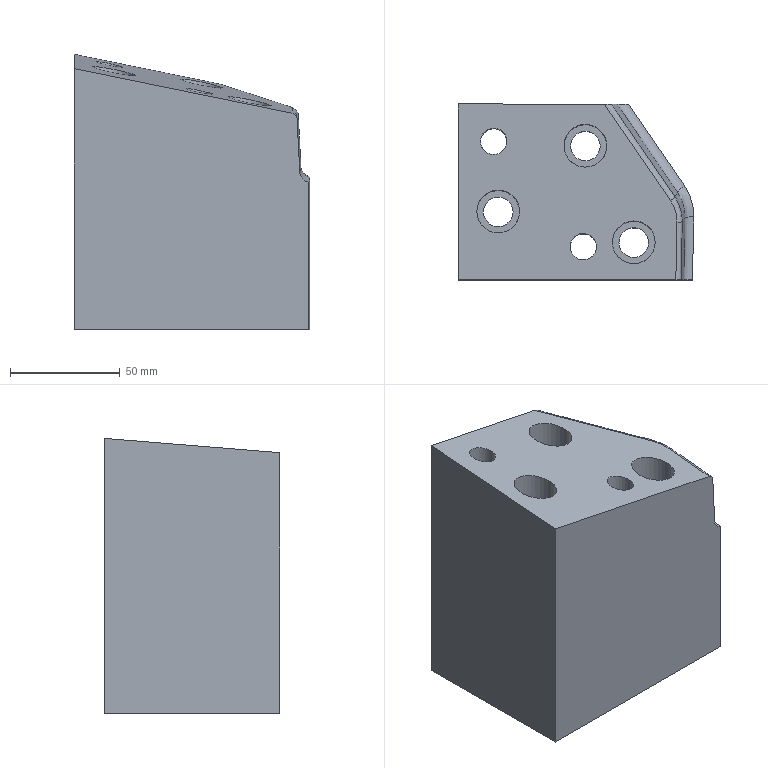Part | NX | features solid 2 | 1 solid | 28 faces | box 107.327 x 80 x 125.43 mm | volume 754575 mm3 | cylinder 10 | spline 9 | plane 9 | commonest cylinder face diameters 13.5 x3 19.5 x3 10 x2 12 x2
STEP:
#1=CARTESIAN_POINT('',(-857.279,-18.669,67.193));
#2=VERTEX_POINT('',#1);
#3=CARTESIAN_POINT('',(-859.902,-22.86,67.388));
#4=CARTESIAN_POINT('',(-856.633,-18.852,67.046));
#5=CARTESIAN_POINT('',(-857.243,-13.746,67.585));
#6=CARTESIAN_POINT('',(-861.169,-10.636,68.641));
#7=CARTESIAN_POINT('',(-866.18,-11.127,69.625));
#8=CARTESIAN_POINT('',(-869.446,-15.132,69.967));
#9=CARTESIAN_POINT('',(-868.843,-20.233,69.429));
#10=CARTESIAN_POINT('',(-864.913,-23.352,68.372));
#11=CARTESIAN_POINT('',(-859.902,-22.86,67.388));
#12=CARTESIAN_POINT('',(-856.633,-18.852,67.046));
#13=CARTESIAN_POINT('',(-857.243,-13.746,67.585));
#14=B_SPLINE_CURVE_WITH_KNOTS('',3,(#3,#4,#5,#6,#7,#8,#9,#10,#11,#12,#13),.UNSPECIFIED.,.T.,.F.,(1,1,1,1,1,1,1,1,1,1,1,1,1,1,1),(-0.01424,-0.009492,-0.004746,0.,0.004746,0.009492,0.01424,0.01898,0.02373,0.02848,0.03322,0.03797,0.04271,0.04746,0.05221),.UNSPECIFIED.);
#15=EDGE_CURVE('',#2,#2,#14,.T.);
#16=ORIENTED_EDGE('',*,*,#15,.F.);
#17=EDGE_LOOP('',(#16));
#18=FACE_BOUND('',#17,.T.);
#19=CARTESIAN_POINT('',(-909.709,-6.673,78.884));
#20=VERTEX_POINT('',#19);
#21=CARTESIAN_POINT('',(-903.612,-11.594,77.238));
#22=CARTESIAN_POINT('',(-910.538,-7.306,79.002));
#23=CARTESIAN_POINT('',(-912.489,0.7824,80.058));
#24=CARTESIAN_POINT('',(-908.008,7.886,79.719));
#25=CARTESIAN_POINT('',(-899.97,9.645,78.219));
#26=CARTESIAN_POINT('',(-893.065,5.359,76.46));
#27=CARTESIAN_POINT('',(-891.101,-2.711,75.402));
#28=CARTESIAN_POINT('',(-895.587,-9.835,75.74));
#29=CARTESIAN_POINT('',(-903.612,-11.594,77.238));
#30=CARTESIAN_POINT('',(-910.538,-7.306,79.002));
#31=CARTESIAN_POINT('',(-912.489,0.7824,80.058));
#32=B_SPLINE_CURVE_WITH_KNOTS('',3,(#21,#22,#23,#24,#25,#26,#27,#28,#29,#30,#31),.UNSPECIFIED.,.T.,.F.,(1,1,1,1,1,1,1,1,1,1,1,1,1,1,1),(-0.02314,-0.01542,-0.007712,0.,0.007712,0.01542,0.02314,0.03085,0.03856,0.04627,0.05398,0.06169,0.06941,0.07712,0.08483),.UNSPECIFIED.);
#33=EDGE_CURVE('',#20,#20,#32,.T.);
#34=ORIENTED_EDGE('',*,*,#33,.T.);
#35=EDGE_LOOP('',(#34));
#36=FACE_BOUND('',#35,.T.);
#37=CARTESIAN_POINT('',(-849.687,-16.103,65.849));
#38=VERTEX_POINT('',#37);
#39=CARTESIAN_POINT('',(-846.7,-23.44,64.643));
#40=CARTESIAN_POINT('',(-850.754,-16.253,66.055));
#41=CARTESIAN_POINT('',(-848.406,-8.168,66.232));
#42=CARTESIAN_POINT('',(-841.091,-4.27,65.054));
#43=CARTESIAN_POINT('',(-833.29,-6.567,63.273));
#44=CARTESIAN_POINT('',(-829.252,-13.743,61.864));
#45=CARTESIAN_POINT('',(-831.581,-21.819,61.684));
#46=CARTESIAN_POINT('',(-838.912,-25.731,62.864));
#47=CARTESIAN_POINT('',(-846.7,-23.44,64.643));
#48=CARTESIAN_POINT('',(-850.754,-16.253,66.055));
#49=CARTESIAN_POINT('',(-848.406,-8.168,66.232));
#50=B_SPLINE_CURVE_WITH_KNOTS('',3,(#39,#40,#41,#42,#43,#44,#45,#46,#47,#48,#49),.UNSPECIFIED.,.T.,.F.,(1,1,1,1,1,1,1,1,1,1,1,1,1,1,1),(-0.02314,-0.01543,-0.007713,0.,0.007713,0.01543,0.02314,0.03085,0.03857,0.04628,0.05399,0.06171,0.06942,0.07713,0.08485),.UNSPECIFIED.);
#51=EDGE_CURVE('',#38,#38,#50,.T.);
#52=ORIENTED_EDGE('',*,*,#51,.T.);
#53=EDGE_LOOP('',(#52));
#54=FACE_BOUND('',#53,.T.);
#55=CARTESIAN_POINT('',(-871.247,25.732,73.656));
#56=VERTEX_POINT('',#55);
#57=CARTESIAN_POINT('',(-866.719,19.289,72.207));
#58=CARTESIAN_POINT('',(-872.237,25.345,73.827));
#59=CARTESIAN_POINT('',(-871.815,33.724,74.421));
#60=CARTESIAN_POINT('',(-865.534,39.227,73.585));
#61=CARTESIAN_POINT('',(-857.389,38.706,71.878));
#62=CARTESIAN_POINT('',(-851.893,32.658,70.263));
#63=CARTESIAN_POINT('',(-852.296,24.292,69.666));
#64=CARTESIAN_POINT('',(-858.589,18.772,70.503));
#65=CARTESIAN_POINT('',(-866.719,19.289,72.207));
#66=CARTESIAN_POINT('',(-872.237,25.345,73.827));
#67=CARTESIAN_POINT('',(-871.815,33.724,74.421));
#68=B_SPLINE_CURVE_WITH_KNOTS('',3,(#57,#58,#59,#60,#61,#62,#63,#64,#65,#66,#67),.UNSPECIFIED.,.T.,.F.,(1,1,1,1,1,1,1,1,1,1,1,1,1,1,1),(-0.02314,-0.01543,-0.007713,0.,0.007713,0.01543,0.02314,0.03085,0.03856,0.04628,0.05399,0.0617,0.06942,0.07713,0.08484),.UNSPECIFIED.);
#69=EDGE_CURVE('',#56,#56,#68,.T.);
#70=ORIENTED_EDGE('',*,*,#69,.T.);
#71=EDGE_LOOP('',(#70));
#72=FACE_BOUND('',#71,.T.);
#73=CARTESIAN_POINT('',(-820.85,-32.,58.663));
#74=VERTEX_POINT('',#73);
#75=CARTESIAN_POINT('',(-920.,-32.,78.929));
#76=VERTEX_POINT('',#75);
#77=CARTESIAN_POINT('',(-820.85,-32.,58.663));
#78=CARTESIAN_POINT('',(-853.9,-32.,65.419));
#79=CARTESIAN_POINT('',(-886.95,-32.,72.174));
#80=CARTESIAN_POINT('',(-920.,-32.,78.929));
#81=B_SPLINE_CURVE_WITH_KNOTS('',3,(#77,#78,#79,#80),.UNSPECIFIED.,.F.,.F.,(4,4),(0.,0.1012),.UNSPECIFIED.);
#82=EDGE_CURVE('',#74,#76,#81,.T.);
#83=ORIENTED_EDGE('',*,*,#82,.F.);
#84=CARTESIAN_POINT('',(-820.322,-5.79,60.685));
#85=VERTEX_POINT('',#84);
#86=CARTESIAN_POINT('',(-820.85,-32.,58.663));
#87=CARTESIAN_POINT('',(-820.674,-23.263,59.337));
#88=CARTESIAN_POINT('',(-820.498,-14.527,60.011));
#89=CARTESIAN_POINT('',(-820.322,-5.79,60.685));
#90=B_SPLINE_CURVE_WITH_KNOTS('',3,(#86,#87,#88,#89),.UNSPECIFIED.,.F.,.F.,(4,4),(-0.002388,0.0239),.UNSPECIFIED.);
#91=EDGE_CURVE('',#74,#85,#90,.T.);
#92=ORIENTED_EDGE('',*,*,#91,.T.);
#93=CARTESIAN_POINT('',(-823.204,3.89,62.061));
#94=VERTEX_POINT('',#93);
#95=CARTESIAN_POINT('',(-820.322,-5.79,60.685));
#96=CARTESIAN_POINT('',(-820.252,-2.334,60.952));
#97=CARTESIAN_POINT('',(-821.278,1.075,61.439));
#98=CARTESIAN_POINT('',(-823.204,3.89,62.061));
#99=B_SPLINE_CURVE_WITH_KNOTS('',3,(#95,#96,#97,#98),.UNSPECIFIED.,.F.,.F.,(4,4),(0.,0.01034),.UNSPECIFIED.);
#100=EDGE_CURVE('',#85,#94,#99,.T.);
#101=ORIENTED_EDGE('',*,*,#100,.T.);
#102=CARTESIAN_POINT('',(-853.376,48.,71.813));
#103=VERTEX_POINT('',#102);
#104=CARTESIAN_POINT('',(-823.204,3.89,62.061));
#105=CARTESIAN_POINT('',(-833.261,18.593,65.312));
#106=CARTESIAN_POINT('',(-843.319,33.297,68.562));
#107=CARTESIAN_POINT('',(-853.376,48.,71.813));
#108=B_SPLINE_CURVE_WITH_KNOTS('',3,(#104,#105,#106,#107),.UNSPECIFIED.,.F.,.F.,(4,4),(0.,0.05432),.UNSPECIFIED.);
#109=EDGE_CURVE('',#94,#103,#108,.T.);
#110=ORIENTED_EDGE('',*,*,#109,.T.);
#111=CARTESIAN_POINT('',(-920.,48.,85.43));
#112=VERTEX_POINT('',#111);
#113=CARTESIAN_POINT('',(-853.376,48.,71.813));
#114=CARTESIAN_POINT('',(-875.584,48.,76.352));
#115=CARTESIAN_POINT('',(-897.792,48.,80.891));
#116=CARTESIAN_POINT('',(-920.,48.,85.43));
#117=B_SPLINE_CURVE_WITH_KNOTS('',3,(#113,#114,#115,#116),.UNSPECIFIED.,.F.,.F.,(4,4),(0.1961,0.2641),.UNSPECIFIED.);
#118=EDGE_CURVE('',#103,#112,#117,.T.);
#119=ORIENTED_EDGE('',*,*,#118,.T.);
#120=CARTESIAN_POINT('',(-920.,-32.,78.929));
#121=CARTESIAN_POINT('',(-920.,-5.333,81.096));
#122=CARTESIAN_POINT('',(-920.,21.333,83.263));
#123=CARTESIAN_POINT('',(-920.,48.,85.43));
#124=B_SPLINE_CURVE_WITH_KNOTS('',3,(#120,#121,#122,#123),.UNSPECIFIED.,.F.,.F.,(4,4),(0.,0.08026),.UNSPECIFIED.);
#125=EDGE_CURVE('',#76,#112,#124,.T.);
#126=ORIENTED_EDGE('',*,*,#125,.F.);
#127=EDGE_LOOP('',(#83,#92,#101,#110,#119,#126));
#128=FACE_BOUND('',#127,.T.);
#129=CARTESIAN_POINT('',(-908.757,34.366,82.024));
#130=VERTEX_POINT('',#129);
#131=CARTESIAN_POINT('',(-904.976,37.499,81.506));
#132=CARTESIAN_POINT('',(-909.304,34.754,82.168));
#133=CARTESIAN_POINT('',(-910.352,29.683,81.97));
#134=CARTESIAN_POINT('',(-907.547,25.48,81.055));
#135=CARTESIAN_POINT('',(-902.655,24.423,79.969));
#136=CARTESIAN_POINT('',(-898.335,27.166,79.309));
#137=CARTESIAN_POINT('',(-897.28,32.228,79.505));
#138=CARTESIAN_POINT('',(-900.089,36.443,80.421));
#139=CARTESIAN_POINT('',(-904.976,37.499,81.506));
#140=CARTESIAN_POINT('',(-909.304,34.754,82.168));
#141=CARTESIAN_POINT('',(-910.352,29.683,81.97));
#142=B_SPLINE_CURVE_WITH_KNOTS('',3,(#131,#132,#133,#134,#135,#136,#137,#138,#139,#140,#141),.UNSPECIFIED.,.T.,.F.,(1,1,1,1,1,1,1,1,1,1,1,1,1,1,1),(-0.01424,-0.009493,-0.004747,0.,0.004747,0.009493,0.01424,0.01899,0.02373,0.02848,0.03323,0.03797,0.04272,0.04747,0.05221),.UNSPECIFIED.);
#143=EDGE_CURVE('',#130,#130,#142,.T.);
#144=ORIENTED_EDGE('',*,*,#143,.F.);
#145=EDGE_LOOP('',(#144));
#146=FACE_BOUND('',#145,.T.);
#147=CARTESIAN_POINT('',(-920.973,48.472,85.668));
#148=CARTESIAN_POINT('',(-920.587,-34.619,78.836));
#149=CARTESIAN_POINT('',(-919.909,48.495,85.452));
#150=CARTESIAN_POINT('',(-919.523,-34.596,78.62));
#151=CARTESIAN_POINT('',(-900.858,48.901,81.591));
#152=CARTESIAN_POINT('',(-900.471,-34.19,74.759));
#153=CARTESIAN_POINT('',(-869.11,49.577,75.157));
#154=CARTESIAN_POINT('',(-868.723,-33.513,68.325));
#155=CARTESIAN_POINT('',(-819.956,50.625,65.195));
#156=CARTESIAN_POINT('',(-819.569,-32.465,58.364));
#157=B_SPLINE_SURFACE_WITH_KNOTS('',1,1,((#147,#148),(#149,#150),(#151,#152),(#153,#154),(#155,#156)),.PLANE_SURF.,.F.,.F.,.F.,(2,1,1,1,2),(2,2),(-0.2849,-0.2791,-0.1744,0.,0.2701),(0.3913,0.7679),.PIECEWISE_BEZIER_KNOTS.);
#158=ADVANCED_FACE('',(#18,#36,#54,#72,#128,#146),#157,.F.);
#159=CARTESIAN_POINT('',(-869.041,-16.993,-40.));
#160=VERTEX_POINT('',#159);
#161=CARTESIAN_POINT('',(-863.041,-16.993,-40.));
#162=DIRECTION('',(0.,0.,-1.));
#163=DIRECTION('',(-1.,0.,0.));
#164=AXIS2_PLACEMENT_3D('',#161,#162,#163);
#165=CIRCLE('',#164,6.);
#166=EDGE_CURVE('',#160,#160,#165,.F.);
#167=ORIENTED_EDGE('',*,*,#166,.T.);
#168=EDGE_LOOP('',(#167));
#169=FACE_BOUND('',#168,.T.);
#170=CARTESIAN_POINT('',(-908.547,-0.9737,-40.));
#171=VERTEX_POINT('',#170);
#172=CARTESIAN_POINT('',(-901.797,-0.9737,-40.));
#173=DIRECTION('',(0.,0.,-1.));
#174=DIRECTION('',(-1.,0.,0.));
#175=AXIS2_PLACEMENT_3D('',#172,#173,#174);
#176=CIRCLE('',#175,6.75);
#177=EDGE_CURVE('',#171,#171,#176,.T.);
#178=ORIENTED_EDGE('',*,*,#177,.F.);
#179=EDGE_LOOP('',(#178));
#180=FACE_BOUND('',#179,.T.);
#181=CARTESIAN_POINT('',(-846.75,-15.,-40.));
#182=VERTEX_POINT('',#181);
#183=CARTESIAN_POINT('',(-840.,-15.,-40.));
#184=DIRECTION('',(0.,0.,-1.));
#185=DIRECTION('',(-1.,0.,0.));
#186=AXIS2_PLACEMENT_3D('',#183,#184,#185);
#187=CIRCLE('',#186,6.75);
#188=EDGE_CURVE('',#182,#182,#187,.T.);
#189=ORIENTED_EDGE('',*,*,#188,.F.);
#190=EDGE_LOOP('',(#189));
#191=FACE_BOUND('',#190,.T.);
#192=CARTESIAN_POINT('',(-868.811,29.,-40.));
#193=VERTEX_POINT('',#192);
#194=CARTESIAN_POINT('',(-862.061,29.,-40.));
#195=DIRECTION('',(0.,0.,-1.));
#196=DIRECTION('',(-1.,0.,0.));
#197=AXIS2_PLACEMENT_3D('',#194,#195,#196);
#198=CIRCLE('',#197,6.75);
#199=EDGE_CURVE('',#193,#193,#198,.T.);
#200=ORIENTED_EDGE('',*,*,#199,.F.);
#201=EDGE_LOOP('',(#200));
#202=FACE_BOUND('',#201,.T.);
#203=CARTESIAN_POINT('',(-813.255,-32.,-40.));
#204=VERTEX_POINT('',#203);
#205=CARTESIAN_POINT('',(-920.,-32.,-40.));
#206=VERTEX_POINT('',#205);
#207=CARTESIAN_POINT('',(-813.69,-32.,-40.));
#208=DIRECTION('',(-1.,0.,0.));
#209=VECTOR('',#208,1000.);
#210=LINE('',#207,#209);
#211=EDGE_CURVE('',#204,#206,#210,.T.);
#212=ORIENTED_EDGE('',*,*,#211,.T.);
#213=CARTESIAN_POINT('',(-920.,48.,-40.));
#214=VERTEX_POINT('',#213);
#215=CARTESIAN_POINT('',(-920.,-31.695,-40.));
#216=DIRECTION('',(0.,1.,0.));
#217=VECTOR('',#216,1000.);
#218=LINE('',#215,#217);
#219=EDGE_CURVE('',#206,#214,#218,.T.);
#220=ORIENTED_EDGE('',*,*,#219,.T.);
#221=CARTESIAN_POINT('',(-842.318,48.,-40.));
#222=VERTEX_POINT('',#221);
#223=CARTESIAN_POINT('',(-813.69,48.,-40.));
#224=DIRECTION('',(1.,0.,0.));
#225=VECTOR('',#224,1000.);
#226=LINE('',#223,#225);
#227=EDGE_CURVE('',#222,#214,#226,.F.);
#228=ORIENTED_EDGE('',*,*,#227,.F.);
#229=CARTESIAN_POINT('',(-816.916,10.864,-40.));
#230=VERTEX_POINT('',#229);
#231=CARTESIAN_POINT('',(-812.737,4.755,-40.));
#232=DIRECTION('',(0.5646,-0.8254,0.));
#233=VECTOR('',#232,1000.);
#234=LINE('',#231,#233);
#235=EDGE_CURVE('',#222,#230,#234,.T.);
#236=ORIENTED_EDGE('',*,*,#235,.T.);
#237=CARTESIAN_POINT('',(-812.678,-3.372,-40.));
#238=VERTEX_POINT('',#237);
#239=CARTESIAN_POINT('',(-812.678,-3.372,-40.));
#240=CARTESIAN_POINT('',(-812.627,-0.8443,-40.));
#241=CARTESIAN_POINT('',(-813.295,4.147,-40.));
#242=CARTESIAN_POINT('',(-815.489,8.778,-40.));
#243=CARTESIAN_POINT('',(-816.916,10.864,-40.));
#244=B_SPLINE_CURVE_WITH_KNOTS('',3,(#239,#240,#241,#242,#243),.UNSPECIFIED.,.F.,.F.,(4,1,4),(0.06077,0.06835,0.07594),.UNSPECIFIED.);
#245=EDGE_CURVE('',#238,#230,#244,.T.);
#246=ORIENTED_EDGE('',*,*,#245,.F.);
#247=CARTESIAN_POINT('',(-812.528,4.08,-40.));
#248=DIRECTION('',(0.02015,0.9998,0.));
#249=VECTOR('',#248,1000.);
#250=LINE('',#247,#249);
#251=EDGE_CURVE('',#204,#238,#250,.T.);
#252=ORIENTED_EDGE('',*,*,#251,.F.);
#253=EDGE_LOOP('',(#212,#220,#228,#236,#246,#252));
#254=FACE_BOUND('',#253,.T.);
#255=CARTESIAN_POINT('',(-909.818,30.961,-40.));
#256=VERTEX_POINT('',#255);
#257=CARTESIAN_POINT('',(-903.818,30.961,-40.));
#258=DIRECTION('',(0.,0.,-1.));
#259=DIRECTION('',(-1.,0.,0.));
#260=AXIS2_PLACEMENT_3D('',#257,#258,#259);
#261=CIRCLE('',#260,6.);
#262=EDGE_CURVE('',#256,#256,#261,.F.);
#263=ORIENTED_EDGE('',*,*,#262,.T.);
#264=EDGE_LOOP('',(#263));
#265=FACE_BOUND('',#264,.T.);
#266=CARTESIAN_POINT('',(-813.69,4.103,-40.));
#267=DIRECTION('',(0.,0.,-1.));
#268=DIRECTION('',(-1.,0.,0.));
#269=AXIS2_PLACEMENT_3D('',#266,#267,#268);
#270=PLANE('',#269);
#271=ADVANCED_FACE('',(#169,#180,#191,#202,#254,#265),#270,.T.);
#272=CARTESIAN_POINT('',(-818.457,-32.,55.871));
#273=VERTEX_POINT('',#272);
#274=CARTESIAN_POINT('',(-817.244,-32.,31.764));
#275=VERTEX_POINT('',#274);
#276=CARTESIAN_POINT('',(-818.457,-32.,55.871));
#277=CARTESIAN_POINT('',(-818.053,-32.,47.836));
#278=CARTESIAN_POINT('',(-817.648,-32.,39.8));
#279=CARTESIAN_POINT('',(-817.244,-32.,31.764));
#280=B_SPLINE_CURVE_WITH_KNOTS('',3,(#276,#277,#278,#279),.UNSPECIFIED.,.F.,.F.,(4,4),(0.06257,0.08671),.UNSPECIFIED.);
#281=EDGE_CURVE('',#273,#275,#280,.T.);
#282=ORIENTED_EDGE('',*,*,#281,.F.);
#283=CARTESIAN_POINT('',(-818.457,-32.,55.871));
#284=CARTESIAN_POINT('',(-818.524,-32.,57.201));
#285=CARTESIAN_POINT('',(-819.546,-32.,58.397));
#286=CARTESIAN_POINT('',(-820.85,-32.,58.663));
#287=B_SPLINE_CURVE_WITH_KNOTS('',3,(#283,#284,#285,#286),.UNSPECIFIED.,.F.,.F.,(4,4),(0.,0.003938),.UNSPECIFIED.);
#288=EDGE_CURVE('',#273,#74,#287,.T.);
#289=ORIENTED_EDGE('',*,*,#288,.T.);
#290=ORIENTED_EDGE('',*,*,#82,.T.);
#291=CARTESIAN_POINT('',(-920.,-32.,100.));
#292=DIRECTION('',(0.,0.,-1.));
#293=VECTOR('',#292,1000.);
#294=LINE('',#291,#293);
#295=EDGE_CURVE('',#76,#206,#294,.T.);
#296=ORIENTED_EDGE('',*,*,#295,.T.);
#297=ORIENTED_EDGE('',*,*,#211,.F.);
#298=CARTESIAN_POINT('',(-813.255,-32.,27.111));
#299=VERTEX_POINT('',#298);
#300=CARTESIAN_POINT('',(-813.255,-32.,-47.5));
#301=DIRECTION('',(0.,0.,-1.));
#302=VECTOR('',#301,1000.);
#303=LINE('',#300,#302);
#304=EDGE_CURVE('',#299,#204,#303,.T.);
#305=ORIENTED_EDGE('',*,*,#304,.F.);
#306=CARTESIAN_POINT('',(-812.249,-32.,32.025));
#307=DIRECTION('',(0.,-1.,0.));
#308=DIRECTION('',(0.2528,0.,0.9675));
#309=AXIS2_PLACEMENT_3D('',#306,#307,#308);
#310=ELLIPSE('',#309,5.016,5.);
#311=EDGE_CURVE('',#299,#275,#310,.F.);
#312=ORIENTED_EDGE('',*,*,#311,.T.);
#313=EDGE_LOOP('',(#282,#289,#290,#296,#297,#305,#312));
#314=FACE_BOUND('',#313,.T.);
#315=CARTESIAN_POINT('',(-915.5,-32.,-47.5));
#316=DIRECTION('',(0.,-1.,0.));
#317=DIRECTION('',(1.,0.,0.));
#318=AXIS2_PLACEMENT_3D('',#315,#316,#317);
#319=PLANE('',#318);
#320=ADVANCED_FACE('',(#314),#319,.T.);
#321=ORIENTED_EDGE('',*,*,#118,.F.);
#322=CARTESIAN_POINT('',(-850.193,48.,68.733));
#323=VERTEX_POINT('',#322);
#324=CARTESIAN_POINT('',(-853.376,48.,71.813));
#325=CARTESIAN_POINT('',(-852.599,48.,71.654));
#326=CARTESIAN_POINT('',(-851.151,48.,70.951));
#327=CARTESIAN_POINT('',(-850.277,48.,69.525));
#328=CARTESIAN_POINT('',(-850.193,48.,68.733));
#329=B_SPLINE_CURVE_WITH_KNOTS('',3,(#324,#325,#326,#327,#328),.UNSPECIFIED.,.F.,.F.,(4,1,4),(0.,0.002346,0.004693),.UNSPECIFIED.);
#330=EDGE_CURVE('',#103,#323,#329,.T.);
#331=ORIENTED_EDGE('',*,*,#330,.T.);
#332=CARTESIAN_POINT('',(-847.625,48.,44.687));
#333=VERTEX_POINT('',#332);
#334=CARTESIAN_POINT('',(-847.625,48.,44.687));
#335=CARTESIAN_POINT('',(-848.481,48.,52.702));
#336=CARTESIAN_POINT('',(-849.337,48.,60.717));
#337=CARTESIAN_POINT('',(-850.193,48.,68.733));
#338=B_SPLINE_CURVE_WITH_KNOTS('',3,(#334,#335,#336,#337),.UNSPECIFIED.,.F.,.F.,(4,4),(0.,0.02418),.UNSPECIFIED.);
#339=EDGE_CURVE('',#333,#323,#338,.T.);
#340=ORIENTED_EDGE('',*,*,#339,.F.);
#341=CARTESIAN_POINT('',(-842.318,48.,39.553));
#342=VERTEX_POINT('',#341);
#343=CARTESIAN_POINT('',(-841.592,48.,44.524));
#344=DIRECTION('',(0.,1.,0.));
#345=DIRECTION('',(0.9515,0.,-0.3075));
#346=AXIS2_PLACEMENT_3D('',#343,#344,#345);
#347=ELLIPSE('',#346,6.158,5.);
#348=EDGE_CURVE('',#342,#333,#347,.T.);
#349=ORIENTED_EDGE('',*,*,#348,.F.);
#350=CARTESIAN_POINT('',(-842.318,48.,100.));
#351=DIRECTION('',(0.,0.,1.));
#352=VECTOR('',#351,1000.);
#353=LINE('',#350,#352);
#354=EDGE_CURVE('',#342,#222,#353,.F.);
#355=ORIENTED_EDGE('',*,*,#354,.T.);
#356=ORIENTED_EDGE('',*,*,#227,.T.);
#357=CARTESIAN_POINT('',(-920.,48.,100.));
#358=DIRECTION('',(0.,0.,1.));
#359=VECTOR('',#358,1000.);
#360=LINE('',#357,#359);
#361=EDGE_CURVE('',#112,#214,#360,.F.);
#362=ORIENTED_EDGE('',*,*,#361,.F.);
#363=EDGE_LOOP('',(#321,#331,#340,#349,#355,#356,#362));
#364=FACE_BOUND('',#363,.T.);
#365=CARTESIAN_POINT('',(-915.5,48.,-47.5));
#366=DIRECTION('',(0.,1.,0.));
#367=DIRECTION('',(-1.,0.,0.));
#368=AXIS2_PLACEMENT_3D('',#365,#366,#367);
#369=PLANE('',#368);
#370=ADVANCED_FACE('',(#364),#369,.T.);
#371=ORIENTED_EDGE('',*,*,#354,.F.);
#372=CARTESIAN_POINT('',(-816.916,10.864,31.343));
#373=VERTEX_POINT('',#372);
#374=CARTESIAN_POINT('',(-842.318,48.,39.553));
#375=CARTESIAN_POINT('',(-833.851,35.621,36.816));
#376=CARTESIAN_POINT('',(-825.383,23.243,34.079));
#377=CARTESIAN_POINT('',(-816.916,10.864,31.343));
#378=B_SPLINE_CURVE_WITH_KNOTS('',3,(#374,#375,#376,#377),.UNSPECIFIED.,.F.,.F.,(4,4),(-0.01765,1.),.UNSPECIFIED.);
#379=EDGE_CURVE('',#342,#373,#378,.T.);
#380=ORIENTED_EDGE('',*,*,#379,.T.);
#381=CARTESIAN_POINT('',(-816.916,10.864,100.));
#382=DIRECTION('',(0.,0.,-1.));
#383=VECTOR('',#382,1000.);
#384=LINE('',#381,#383);
#385=EDGE_CURVE('',#373,#230,#384,.T.);
#386=ORIENTED_EDGE('',*,*,#385,.T.);
#387=ORIENTED_EDGE('',*,*,#235,.F.);
#388=EDGE_LOOP('',(#371,#380,#386,#387));
#389=FACE_BOUND('',#388,.T.);
#390=CARTESIAN_POINT('',(-841.878,47.356,100.));
#391=DIRECTION('',(0.8254,0.5646,0.));
#392=DIRECTION('',(-0.5646,0.8254,0.));
#393=AXIS2_PLACEMENT_3D('',#390,#391,#392);
#394=PLANE('',#393);
#395=ADVANCED_FACE('',(#389),#394,.T.);
#396=CARTESIAN_POINT('',(-812.678,-3.372,29.32));
#397=VERTEX_POINT('',#396);
#398=CARTESIAN_POINT('',(-813.255,-32.,27.111));
#399=CARTESIAN_POINT('',(-813.063,-22.457,27.847));
#400=CARTESIAN_POINT('',(-812.87,-12.914,28.583));
#401=CARTESIAN_POINT('',(-812.678,-3.372,29.32));
#402=B_SPLINE_CURVE_WITH_KNOTS('',3,(#398,#399,#400,#401),.UNSPECIFIED.,.F.,.F.,(4,4),(-0.0907,1.),.UNSPECIFIED.);
#403=EDGE_CURVE('',#299,#397,#402,.T.);
#404=ORIENTED_EDGE('',*,*,#403,.F.);
#405=ORIENTED_EDGE('',*,*,#304,.T.);
#406=ORIENTED_EDGE('',*,*,#251,.T.);
#407=CARTESIAN_POINT('',(-812.678,-3.372,100.));
#408=DIRECTION('',(0.,0.,-1.));
#409=VECTOR('',#408,1000.);
#410=LINE('',#407,#409);
#411=EDGE_CURVE('',#397,#238,#410,.T.);
#412=ORIENTED_EDGE('',*,*,#411,.F.);
#413=EDGE_LOOP('',(#404,#405,#406,#412));
#414=FACE_BOUND('',#413,.T.);
#415=CARTESIAN_POINT('',(-813.207,-29.619,100.));
#416=DIRECTION('',(-0.9998,0.02015,0.));
#417=DIRECTION('',(-0.02015,-0.9998,0.));
#418=AXIS2_PLACEMENT_3D('',#415,#416,#417);
#419=PLANE('',#418);
#420=ADVANCED_FACE('',(#414),#419,.F.);
#421=ORIENTED_EDGE('',*,*,#219,.F.);
#422=ORIENTED_EDGE('',*,*,#295,.F.);
#423=ORIENTED_EDGE('',*,*,#125,.T.);
#424=ORIENTED_EDGE('',*,*,#361,.T.);
#425=EDGE_LOOP('',(#421,#422,#423,#424));
#426=FACE_BOUND('',#425,.T.);
#427=CARTESIAN_POINT('',(-920.,-31.695,100.));
#428=DIRECTION('',(1.,0.,0.));
#429=DIRECTION('',(0.,0.,1.));
#430=AXIS2_PLACEMENT_3D('',#427,#428,#429);
#431=PLANE('',#430);
#432=ADVANCED_FACE('',(#426),#431,.F.);
#433=ORIENTED_EDGE('',*,*,#385,.F.);
#434=CARTESIAN_POINT('',(-816.916,10.864,31.343));
#435=CARTESIAN_POINT('',(-813.844,6.373,30.35));
#436=CARTESIAN_POINT('',(-812.585,1.24,29.675));
#437=CARTESIAN_POINT('',(-812.678,-3.372,29.32));
#438=B_SPLINE_CURVE_WITH_KNOTS('',3,(#434,#435,#436,#437),.UNSPECIFIED.,.F.,.F.,(4,4),(0.,1.),.UNSPECIFIED.);
#439=EDGE_CURVE('',#373,#397,#438,.T.);
#440=ORIENTED_EDGE('',*,*,#439,.T.);
#441=ORIENTED_EDGE('',*,*,#411,.T.);
#442=ORIENTED_EDGE('',*,*,#245,.T.);
#443=EDGE_LOOP('',(#433,#440,#441,#442));
#444=FACE_BOUND('',#443,.T.);
#445=CARTESIAN_POINT('',(-812.678,-3.372,31.771));
#446=CARTESIAN_POINT('',(-812.678,-3.372,-40.));
#447=CARTESIAN_POINT('',(-812.576,1.691,31.771));
#448=CARTESIAN_POINT('',(-812.576,1.691,-40.));
#449=CARTESIAN_POINT('',(-814.095,6.74,31.771));
#450=CARTESIAN_POINT('',(-814.095,6.74,-40.));
#451=CARTESIAN_POINT('',(-816.916,10.864,31.771));
#452=CARTESIAN_POINT('',(-816.916,10.864,-40.));
#453=B_SPLINE_SURFACE_WITH_KNOTS('',3,1,((#445,#446),(#447,#448),(#449,#450),(#451,#452)),.SURF_OF_LINEAR_EXTRUSION.,.F.,.F.,.F.,(4,4),(2,2),(0.,1.),(0.,1.),.PIECEWISE_BEZIER_KNOTS.);
#454=ADVANCED_FACE('',(#444),#453,.F.);
#455=ORIENTED_EDGE('',*,*,#348,.T.);
#456=CARTESIAN_POINT('',(-844.632,43.625,43.72));
#457=VERTEX_POINT('',#456);
#458=CARTESIAN_POINT('',(-813.552,-1.812,33.674));
#459=DIRECTION('',(0.5554,-0.812,-0.1795));
#460=VECTOR('',#459,1000.);
#461=LINE('',#458,#460);
#462=EDGE_CURVE('',#457,#333,#461,.F.);
#463=ORIENTED_EDGE('',*,*,#462,.F.);
#464=CARTESIAN_POINT('',(-820.074,7.722,35.782));
#465=VERTEX_POINT('',#464);
#466=CARTESIAN_POINT('',(-820.074,7.722,35.782));
#467=CARTESIAN_POINT('',(-828.26,19.69,38.428));
#468=CARTESIAN_POINT('',(-836.446,31.657,41.074));
#469=CARTESIAN_POINT('',(-844.632,43.625,43.72));
#470=B_SPLINE_CURVE_WITH_KNOTS('',3,(#466,#467,#468,#469),.UNSPECIFIED.,.F.,.F.,(4,4),(0.,1.),.UNSPECIFIED.);
#471=EDGE_CURVE('',#465,#457,#470,.T.);
#472=ORIENTED_EDGE('',*,*,#471,.F.);
#473=CARTESIAN_POINT('',(-816.916,10.864,31.343));
#474=CARTESIAN_POINT('',(-817.831,10.208,31.476));
#475=CARTESIAN_POINT('',(-819.497,8.836,32.526));
#476=CARTESIAN_POINT('',(-820.104,7.947,34.672));
#477=CARTESIAN_POINT('',(-820.074,7.722,35.782));
#478=B_SPLINE_CURVE_WITH_KNOTS('',3,(#473,#474,#475,#476,#477),.UNSPECIFIED.,.F.,.F.,(4,1,4),(0.,0.5,1.),.UNSPECIFIED.);
#479=EDGE_CURVE('',#465,#373,#478,.F.);
#480=ORIENTED_EDGE('',*,*,#479,.T.);
#481=ORIENTED_EDGE('',*,*,#379,.F.);
#482=EDGE_LOOP('',(#455,#463,#472,#480,#481));
#483=FACE_BOUND('',#482,.T.);
#484=CARTESIAN_POINT('',(-809.396,0.9322,34.118));
#485=DIRECTION('',(0.5554,-0.812,-0.1795));
#486=DIRECTION('',(-0.8312,-0.5489,-0.08875));
#487=AXIS2_PLACEMENT_3D('',#484,#485,#486);
#488=CYLINDRICAL_SURFACE('',#487,5.);
#489=ADVANCED_FACE('',(#483),#488,.F.);
#490=CARTESIAN_POINT('',(-821.309,5.775,59.397));
#491=VERTEX_POINT('',#490);
#492=CARTESIAN_POINT('',(-819.624,8.431,27.186));
#493=CARTESIAN_POINT('',(-819.845,8.082,31.423));
#494=CARTESIAN_POINT('',(-820.016,7.813,34.682));
#495=CARTESIAN_POINT('',(-821.153,6.021,56.409));
#496=CARTESIAN_POINT('',(-821.323,5.753,59.668));
#497=CARTESIAN_POINT('',(-821.545,5.403,63.905));
#498=(BOUNDED_CURVE()B_SPLINE_CURVE(1,(#492,#493,#494,#495,#496,#497),.UNSPECIFIED.,.F.,.F.)B_SPLINE_CURVE_WITH_KNOTS((2,1,1,1,1,2),(-0.345,-0.15,0.,1.,1.15,1.345),.PIECEWISE_BEZIER_KNOTS.)CURVE()GEOMETRIC_REPRESENTATION_ITEM()RATIONAL_B_SPLINE_CURVE((1.,1.,1.,1.,1.,1.))REPRESENTATION_ITEM(''));
#499=EDGE_CURVE('',#465,#491,#498,.T.);
#500=ORIENTED_EDGE('',*,*,#499,.T.);
#501=CARTESIAN_POINT('',(-817.926,-5.624,57.906));
#502=VERTEX_POINT('',#501);
#503=CARTESIAN_POINT('',(-821.309,5.775,59.397));
#504=CARTESIAN_POINT('',(-819.061,2.474,58.755));
#505=CARTESIAN_POINT('',(-817.844,-1.592,58.221));
#506=CARTESIAN_POINT('',(-817.926,-5.624,57.906));
#507=B_SPLINE_CURVE_WITH_KNOTS('',3,(#503,#504,#505,#506),.UNSPECIFIED.,.F.,.F.,(4,4),(-0.00000006,0.01214),.UNSPECIFIED.);
#508=EDGE_CURVE('',#491,#502,#507,.T.);
#509=ORIENTED_EDGE('',*,*,#508,.T.);
#510=CARTESIAN_POINT('',(-816.672,-3.648,33.952));
#511=VERTEX_POINT('',#510);
#512=CARTESIAN_POINT('',(-818.227,-6.099,63.671));
#513=CARTESIAN_POINT('',(-817.961,-5.679,58.575));
#514=CARTESIAN_POINT('',(-817.755,-5.356,54.656));
#515=CARTESIAN_POINT('',(-817.598,-5.107,51.641));
#516=CARTESIAN_POINT('',(-817.476,-4.916,49.322));
#517=CARTESIAN_POINT('',(-816.667,-3.641,33.86));
#518=CARTESIAN_POINT('',(-816.546,-3.45,31.541));
#519=CARTESIAN_POINT('',(-816.388,-3.201,28.526));
#520=CARTESIAN_POINT('',(-816.183,-2.878,24.606));
#521=CARTESIAN_POINT('',(-815.917,-2.458,19.511));
#522=B_SPLINE_CURVE_WITH_KNOTS('',1,(#512,#513,#514,#515,#516,#517,#518,#519,#520,#521),.UNSPECIFIED.,.F.,.F.,(2,1,1,1,1,1,1,1,1,2),(-0.9281,-0.5985,-0.345,-0.15,0.,1.,1.15,1.345,1.599,1.928),.PIECEWISE_BEZIER_KNOTS.);
#523=EDGE_CURVE('',#502,#511,#522,.T.);
#524=ORIENTED_EDGE('',*,*,#523,.T.);
#525=CARTESIAN_POINT('',(-816.672,-3.648,33.952));
#526=CARTESIAN_POINT('',(-816.595,0.1523,34.239));
#527=CARTESIAN_POINT('',(-817.731,4.321,34.88));
#528=CARTESIAN_POINT('',(-820.074,7.722,35.782));
#529=B_SPLINE_CURVE_WITH_KNOTS('',3,(#525,#526,#527,#528),.UNSPECIFIED.,.F.,.F.,(4,4),(0.,1.),.UNSPECIFIED.);
#530=EDGE_CURVE('',#511,#465,#529,.T.);
#531=ORIENTED_EDGE('',*,*,#530,.T.);
#532=EDGE_LOOP('',(#500,#509,#524,#531));
#533=FACE_BOUND('',#532,.T.);
#534=CARTESIAN_POINT('',(-816.67,-3.645,33.912));
#535=CARTESIAN_POINT('',(-817.807,-5.437,55.639));
#536=CARTESIAN_POINT('',(-818.091,-5.885,61.067));
#537=CARTESIAN_POINT('',(-816.589,0.4523,34.254));
#538=CARTESIAN_POINT('',(-817.726,-1.339,55.981));
#539=CARTESIAN_POINT('',(-818.01,-1.787,61.409));
#540=CARTESIAN_POINT('',(-817.739,4.392,34.519));
#541=CARTESIAN_POINT('',(-818.876,2.6,56.246));
#542=CARTESIAN_POINT('',(-819.16,2.153,61.674));
#543=CARTESIAN_POINT('',(-820.016,7.813,34.682));
#544=CARTESIAN_POINT('',(-821.153,6.021,56.409));
#545=CARTESIAN_POINT('',(-821.437,5.574,61.837));
#546=(BOUNDED_SURFACE()B_SPLINE_SURFACE(3,1,((#534,#535,#536),(#537,#538,#539),(#540,#541,#542),(#543,#544,#545)),.CYLINDRICAL_SURF.,.F.,.F.,.F.)B_SPLINE_SURFACE_WITH_KNOTS((4,4),(2,1,2),(0.,1.),(0.,1.,1.25),.PIECEWISE_BEZIER_KNOTS.)GEOMETRIC_REPRESENTATION_ITEM()RATIONAL_B_SPLINE_SURFACE(((1.,1.,1.),(0.9695,0.9695,0.9695),(0.9695,0.9695,0.9695),(1.,1.,1.)))REPRESENTATION_ITEM('')SURFACE());
#547=ADVANCED_FACE('',(#533),#546,.T.);
#548=ORIENTED_EDGE('',*,*,#339,.T.);
#549=CARTESIAN_POINT('',(-850.193,48.,68.733));
#550=CARTESIAN_POINT('',(-840.565,33.925,65.621));
#551=CARTESIAN_POINT('',(-830.937,19.85,62.509));
#552=CARTESIAN_POINT('',(-821.309,5.775,59.397));
#553=B_SPLINE_CURVE_WITH_KNOTS('',3,(#549,#550,#551,#552),.UNSPECIFIED.,.F.,.F.,(4,4),(-0.0007932,0.05121),.UNSPECIFIED.);
#554=EDGE_CURVE('',#323,#491,#553,.T.);
#555=ORIENTED_EDGE('',*,*,#554,.T.);
#556=ORIENTED_EDGE('',*,*,#499,.F.);
#557=ORIENTED_EDGE('',*,*,#471,.T.);
#558=ORIENTED_EDGE('',*,*,#462,.T.);
#559=EDGE_LOOP('',(#548,#555,#556,#557,#558));
#560=FACE_BOUND('',#559,.T.);
#561=CARTESIAN_POINT('',(-867.437,63.159,136.471));
#562=CARTESIAN_POINT('',(-862.32,71.224,38.668));
#563=CARTESIAN_POINT('',(-865.871,60.805,136.359));
#564=CARTESIAN_POINT('',(-860.753,68.87,38.556));
#565=CARTESIAN_POINT('',(-856.814,47.197,135.711));
#566=CARTESIAN_POINT('',(-851.697,55.262,37.907));
#567=CARTESIAN_POINT('',(-856.442,46.638,135.684));
#568=CARTESIAN_POINT('',(-851.325,54.703,37.881));
#569=CARTESIAN_POINT('',(-825.184,-0.3314,133.446));
#570=CARTESIAN_POINT('',(-820.066,7.734,35.643));
#571=B_SPLINE_SURFACE_WITH_KNOTS('',1,1,((#561,#562),(#563,#564),(#565,#566),(#567,#568),(#569,#570)),.PLANE_SURF.,.F.,.F.,.F.,(2,1,1,1,2),(2,2),(-0.7436,-0.6789,-0.3052,-0.2899,1.),(-3.166,1.),.PIECEWISE_BEZIER_KNOTS.);
#572=ADVANCED_FACE('',(#560),#571,.T.);
#573=ORIENTED_EDGE('',*,*,#523,.F.);
#574=CARTESIAN_POINT('',(-817.926,-5.624,57.906));
#575=CARTESIAN_POINT('',(-818.103,-14.416,57.228));
#576=CARTESIAN_POINT('',(-818.28,-23.208,56.55));
#577=CARTESIAN_POINT('',(-818.457,-32.,55.871));
#578=B_SPLINE_CURVE_WITH_KNOTS('',3,(#574,#575,#576,#577),.UNSPECIFIED.,.F.,.F.,(4,4),(0.,0.02646),.UNSPECIFIED.);
#579=EDGE_CURVE('',#502,#273,#578,.T.);
#580=ORIENTED_EDGE('',*,*,#579,.T.);
#581=ORIENTED_EDGE('',*,*,#281,.T.);
#582=CARTESIAN_POINT('',(-817.188,-29.256,31.976));
#583=VERTEX_POINT('',#582);
#584=CARTESIAN_POINT('',(-817.,-19.93,32.695));
#585=DIRECTION('',(0.02009,0.9968,0.07691));
#586=VECTOR('',#585,1000.);
#587=LINE('',#584,#586);
#588=EDGE_CURVE('',#583,#275,#587,.F.);
#589=ORIENTED_EDGE('',*,*,#588,.F.);
#590=CARTESIAN_POINT('',(-817.185,-29.103,31.988));
#591=VERTEX_POINT('',#590);
#592=CARTESIAN_POINT('',(-817.188,-29.256,31.976));
#593=CARTESIAN_POINT('',(-817.187,-29.205,31.98));
#594=CARTESIAN_POINT('',(-817.186,-29.154,31.984));
#595=CARTESIAN_POINT('',(-817.185,-29.103,31.988));
#596=B_SPLINE_CURVE_WITH_KNOTS('',3,(#592,#593,#594,#595),.UNSPECIFIED.,.F.,.F.,(4,4),(0.,1.),.UNSPECIFIED.);
#597=EDGE_CURVE('',#591,#583,#596,.F.);
#598=ORIENTED_EDGE('',*,*,#597,.F.);
#599=CARTESIAN_POINT('',(-817.185,-29.103,31.988));
#600=CARTESIAN_POINT('',(-817.014,-20.618,32.642));
#601=CARTESIAN_POINT('',(-816.843,-12.133,33.297));
#602=CARTESIAN_POINT('',(-816.672,-3.648,33.952));
#603=B_SPLINE_CURVE_WITH_KNOTS('',3,(#599,#600,#601,#602),.UNSPECIFIED.,.F.,.F.,(4,4),(0.,1.),.UNSPECIFIED.);
#604=EDGE_CURVE('',#511,#591,#603,.F.);
#605=ORIENTED_EDGE('',*,*,#604,.F.);
#606=EDGE_LOOP('',(#573,#580,#581,#589,#598,#605));
#607=FACE_BOUND('',#606,.T.);
#608=CARTESIAN_POINT('',(-821.862,-47.996,115.873));
#609=CARTESIAN_POINT('',(-817.408,-40.976,30.742));
#610=CARTESIAN_POINT('',(-821.122,-10.661,118.99));
#611=CARTESIAN_POINT('',(-816.667,-3.641,33.86));
#612=B_SPLINE_SURFACE_WITH_KNOTS('',1,1,((#608,#609),(#610,#611)),.PLANE_SURF.,.F.,.F.,.F.,(2,2),(2,2),(-0.4588,1.),(-4.506,1.),.UNSPECIFIED.);
#613=ADVANCED_FACE('',(#607),#612,.F.);
#614=CARTESIAN_POINT('',(-816.672,-3.648,33.952));
#615=CARTESIAN_POINT('',(-816.615,-3.565,32.858));
#616=CARTESIAN_POINT('',(-815.752,-3.417,30.713));
#617=CARTESIAN_POINT('',(-813.754,-3.367,29.54));
#618=CARTESIAN_POINT('',(-812.678,-3.372,29.32));
#619=B_SPLINE_CURVE_WITH_KNOTS('',3,(#614,#615,#616,#617,#618),.UNSPECIFIED.,.F.,.F.,(4,1,4),(0.,0.5,1.),.UNSPECIFIED.);
#620=EDGE_CURVE('',#511,#397,#619,.T.);
#621=ORIENTED_EDGE('',*,*,#620,.T.);
#622=ORIENTED_EDGE('',*,*,#439,.F.);
#623=ORIENTED_EDGE('',*,*,#479,.F.);
#624=ORIENTED_EDGE('',*,*,#530,.F.);
#625=EDGE_LOOP('',(#621,#622,#623,#624));
#626=FACE_BOUND('',#625,.T.);
#627=CARTESIAN_POINT('',(-816.916,10.864,31.343));
#628=CARTESIAN_POINT('',(-817.465,10.47,31.423));
#629=CARTESIAN_POINT('',(-817.991,10.068,31.616));
#630=CARTESIAN_POINT('',(-818.473,9.672,31.919));
#631=CARTESIAN_POINT('',(-819.309,8.922,32.721));
#632=CARTESIAN_POINT('',(-819.839,8.313,33.84));
#633=CARTESIAN_POINT('',(-820.013,8.056,34.46));
#634=CARTESIAN_POINT('',(-820.092,7.857,35.116));
#635=CARTESIAN_POINT('',(-820.074,7.722,35.782));
#636=CARTESIAN_POINT('',(-815.226,8.393,30.796));
#637=CARTESIAN_POINT('',(-815.814,8.072,30.891));
#638=CARTESIAN_POINT('',(-816.38,7.742,31.095));
#639=CARTESIAN_POINT('',(-816.901,7.415,31.406));
#640=CARTESIAN_POINT('',(-817.813,6.793,32.217));
#641=CARTESIAN_POINT('',(-818.408,6.276,33.333));
#642=CARTESIAN_POINT('',(-818.613,6.054,33.949));
#643=CARTESIAN_POINT('',(-818.716,5.878,34.6));
#644=CARTESIAN_POINT('',(-818.717,5.753,35.26));
#645=CARTESIAN_POINT('',(-813.909,5.652,30.305));
#646=CARTESIAN_POINT('',(-814.527,5.408,30.411));
#647=CARTESIAN_POINT('',(-815.123,5.156,30.625));
#648=CARTESIAN_POINT('',(-815.674,4.904,30.944));
#649=CARTESIAN_POINT('',(-816.644,4.418,31.765));
#650=CARTESIAN_POINT('',(-817.291,4.005,32.882));
#651=CARTESIAN_POINT('',(-817.519,3.824,33.497));
#652=CARTESIAN_POINT('',(-817.642,3.676,34.144));
#653=CARTESIAN_POINT('',(-817.66,3.565,34.8));
#654=CARTESIAN_POINT('',(-813.026,2.71,29.885));
#655=CARTESIAN_POINT('',(-813.664,2.547,30.002));
#656=CARTESIAN_POINT('',(-814.279,2.376,30.226));
#657=CARTESIAN_POINT('',(-814.85,2.202,30.552));
#658=CARTESIAN_POINT('',(-815.859,1.861,31.384));
#659=CARTESIAN_POINT('',(-816.541,1.558,32.505));
#660=CARTESIAN_POINT('',(-816.784,1.423,33.12));
#661=CARTESIAN_POINT('',(-816.922,1.307,33.766));
#662=CARTESIAN_POINT('',(-816.951,1.215,34.42));
#663=CARTESIAN_POINT('',(-812.617,-0.3319,29.554));
#664=CARTESIAN_POINT('',(-813.264,-0.4118,29.68));
#665=CARTESIAN_POINT('',(-813.889,-0.5004,29.911));
#666=CARTESIAN_POINT('',(-814.469,-0.5946,30.244));
#667=CARTESIAN_POINT('',(-815.496,-0.7875,31.088));
#668=CARTESIAN_POINT('',(-816.193,-0.9754,32.216));
#669=CARTESIAN_POINT('',(-816.444,-1.065,32.834));
#670=CARTESIAN_POINT('',(-816.588,-1.146,33.481));
#671=CARTESIAN_POINT('',(-816.623,-1.216,34.135));
#672=CARTESIAN_POINT('',(-812.678,-3.372,29.32));
#673=CARTESIAN_POINT('',(-813.324,-3.369,29.452));
#674=CARTESIAN_POINT('',(-813.947,-3.375,29.69));
#675=CARTESIAN_POINT('',(-814.526,-3.389,30.029));
#676=CARTESIAN_POINT('',(-815.55,-3.435,30.885));
#677=CARTESIAN_POINT('',(-816.246,-3.508,32.023));
#678=CARTESIAN_POINT('',(-816.495,-3.551,32.645));
#679=CARTESIAN_POINT('',(-816.638,-3.599,33.295));
#680=CARTESIAN_POINT('',(-816.672,-3.648,33.952));
#681=B_SPLINE_SURFACE_WITH_KNOTS('',5,5,((#627,#628,#629,#630,#631,#632,#633,#634,#635),(#636,#637,#638,#639,#640,#641,#642,#643,#644),(#645,#646,#647,#648,#649,#650,#651,#652,#653),(#654,#655,#656,#657,#658,#659,#660,#661,#662),(#663,#664,#665,#666,#667,#668,#669,#670,#671),(#672,#673,#674,#675,#676,#677,#678,#679,#680)),.UNSPECIFIED.,.F.,.F.,.F.,(6,6),(6,3,6),(0.,1.),(0.,0.5,1.),.UNSPECIFIED.);
#682=ADVANCED_FACE('',(#626),#681,.F.);
#683=ORIENTED_EDGE('',*,*,#403,.T.);
#684=ORIENTED_EDGE('',*,*,#620,.F.);
#685=ORIENTED_EDGE('',*,*,#604,.T.);
#686=ORIENTED_EDGE('',*,*,#597,.T.);
#687=ORIENTED_EDGE('',*,*,#588,.T.);
#688=ORIENTED_EDGE('',*,*,#311,.F.);
#689=EDGE_LOOP('',(#683,#684,#685,#686,#687,#688));
#690=FACE_BOUND('',#689,.T.);
#691=CARTESIAN_POINT('',(-812.008,-20.05,32.947));
#692=DIRECTION('',(0.02009,0.9968,0.07691));
#693=DIRECTION('',(0.9984,-0.024,0.05026));
#694=AXIS2_PLACEMENT_3D('',#691,#692,#693);
#695=CYLINDRICAL_SURFACE('',#694,5.);
#696=ADVANCED_FACE('',(#690),#695,.F.);
#697=ORIENTED_EDGE('',*,*,#330,.F.);
#698=ORIENTED_EDGE('',*,*,#109,.F.);
#699=CARTESIAN_POINT('',(-823.803,4.128,59.131));
#700=DIRECTION('',(0.5554,-0.812,-0.1795));
#701=DIRECTION('',(0.8254,0.5646,0.));
#702=AXIS2_PLACEMENT_3D('',#699,#700,#701);
#703=CIRCLE('',#702,3.);
#704=EDGE_CURVE('',#491,#94,#703,.T.);
#705=ORIENTED_EDGE('',*,*,#704,.F.);
#706=ORIENTED_EDGE('',*,*,#554,.F.);
#707=EDGE_LOOP('',(#697,#698,#705,#706));
#708=FACE_BOUND('',#707,.T.);
#709=CARTESIAN_POINT('',(-821.309,5.775,59.397));
#710=CARTESIAN_POINT('',(-821.245,5.293,61.775));
#711=CARTESIAN_POINT('',(-823.204,3.89,62.061));
#712=CARTESIAN_POINT('',(-831.427,20.566,62.668));
#713=CARTESIAN_POINT('',(-831.363,20.085,65.045));
#714=CARTESIAN_POINT('',(-833.322,18.682,65.331));
#715=CARTESIAN_POINT('',(-841.545,35.358,65.938));
#716=CARTESIAN_POINT('',(-841.481,34.876,68.315));
#717=CARTESIAN_POINT('',(-843.44,33.473,68.601));
#718=CARTESIAN_POINT('',(-851.663,50.15,69.208));
#719=CARTESIAN_POINT('',(-851.599,49.668,71.585));
#720=CARTESIAN_POINT('',(-853.558,48.265,71.872));
#721=(BOUNDED_SURFACE()B_SPLINE_SURFACE(3,2,((#709,#710,#711),(#712,#713,#714),(#715,#716,#717),(#718,#719,#720)),.UNSPECIFIED.,.F.,.F.,.F.)B_SPLINE_SURFACE_WITH_KNOTS((4,4),(3,3),(0.02823,0.08288),(0.,1.),.PIECEWISE_BEZIER_KNOTS.)GEOMETRIC_REPRESENTATION_ITEM()RATIONAL_B_SPLINE_SURFACE(((1.,0.7775,1.),(1.,0.7775,1.),(1.,0.7775,1.),(1.,0.7775,1.)))REPRESENTATION_ITEM('')SURFACE());
#722=ADVANCED_FACE('',(#708),#721,.T.);
#723=ORIENTED_EDGE('',*,*,#704,.T.);
#724=ORIENTED_EDGE('',*,*,#100,.F.);
#725=CARTESIAN_POINT('',(-820.921,-5.552,57.756));
#726=DIRECTION('',(-0.02009,-0.9968,-0.07691));
#727=DIRECTION('',(0.,0.07692,-0.997));
#728=AXIS2_PLACEMENT_3D('',#725,#726,#727);
#729=CIRCLE('',#728,3.);
#730=EDGE_CURVE('',#502,#85,#729,.T.);
#731=ORIENTED_EDGE('',*,*,#730,.F.);
#732=ORIENTED_EDGE('',*,*,#508,.F.);
#733=EDGE_LOOP('',(#723,#724,#731,#732));
#734=FACE_BOUND('',#733,.T.);
#735=CARTESIAN_POINT('',(-817.926,-5.624,57.906));
#736=CARTESIAN_POINT('',(-818.046,-5.8,60.219));
#737=CARTESIAN_POINT('',(-820.322,-5.79,60.685));
#738=CARTESIAN_POINT('',(-817.844,-1.558,58.224));
#739=CARTESIAN_POINT('',(-817.97,-1.858,60.524));
#740=CARTESIAN_POINT('',(-820.252,-2.334,60.952));
#741=CARTESIAN_POINT('',(-819.049,2.457,58.751));
#742=CARTESIAN_POINT('',(-819.126,2.072,61.08));
#743=CARTESIAN_POINT('',(-821.278,1.075,61.439));
#744=CARTESIAN_POINT('',(-821.309,5.775,59.397));
#745=CARTESIAN_POINT('',(-821.245,5.293,61.775));
#746=CARTESIAN_POINT('',(-823.204,3.89,62.061));
#747=(BOUNDED_SURFACE()B_SPLINE_SURFACE(3,2,((#735,#736,#737),(#738,#739,#740),(#741,#742,#743),(#744,#745,#746)),.UNSPECIFIED.,.F.,.F.,.F.)B_SPLINE_SURFACE_WITH_KNOTS((4,4),(3,3),(0.,0.01034),(0.,1.),.PIECEWISE_BEZIER_KNOTS.)GEOMETRIC_REPRESENTATION_ITEM()RATIONAL_B_SPLINE_SURFACE(((1.,0.7907,1.),(1.,0.7911,1.),(1.,0.7865,1.),(1.,0.7775,1.)))REPRESENTATION_ITEM('')SURFACE());
#748=ADVANCED_FACE('',(#734),#747,.T.);
#749=ORIENTED_EDGE('',*,*,#288,.F.);
#750=ORIENTED_EDGE('',*,*,#579,.F.);
#751=ORIENTED_EDGE('',*,*,#730,.T.);
#752=ORIENTED_EDGE('',*,*,#91,.F.);
#753=EDGE_LOOP('',(#749,#750,#751,#752));
#754=FACE_BOUND('',#753,.T.);
#755=CARTESIAN_POINT('',(-818.46,-32.158,55.859));
#756=CARTESIAN_POINT('',(-818.581,-32.334,58.172));
#757=CARTESIAN_POINT('',(-820.857,-32.324,58.638));
#758=CARTESIAN_POINT('',(-818.282,-23.313,56.542));
#759=CARTESIAN_POINT('',(-818.403,-23.489,58.855));
#760=CARTESIAN_POINT('',(-820.679,-23.48,59.321));
#761=CARTESIAN_POINT('',(-818.104,-14.469,57.224));
#762=CARTESIAN_POINT('',(-818.224,-14.645,59.537));
#763=CARTESIAN_POINT('',(-820.5,-14.635,60.003));
#764=CARTESIAN_POINT('',(-817.926,-5.624,57.906));
#765=CARTESIAN_POINT('',(-818.046,-5.8,60.219));
#766=CARTESIAN_POINT('',(-820.322,-5.79,60.685));
#767=(BOUNDED_SURFACE()B_SPLINE_SURFACE(3,2,((#755,#756,#757),(#758,#759,#760),(#761,#762,#763),(#764,#765,#766)),.UNSPECIFIED.,.F.,.F.,.F.)B_SPLINE_SURFACE_WITH_KNOTS((4,4),(3,3),(0.01085,0.03747),(0.,1.),.PIECEWISE_BEZIER_KNOTS.)GEOMETRIC_REPRESENTATION_ITEM()RATIONAL_B_SPLINE_SURFACE(((1.,0.7907,1.),(1.,0.7907,1.),(1.,0.7907,1.),(1.,0.7907,1.)))REPRESENTATION_ITEM('')SURFACE());
#768=ADVANCED_FACE('',(#754),#767,.T.);
#769=CARTESIAN_POINT('',(-871.811,29.,-25.));
#770=VERTEX_POINT('',#769);
#771=CARTESIAN_POINT('',(-862.061,29.,-25.));
#772=DIRECTION('',(0.,0.,-1.));
#773=DIRECTION('',(-1.,0.,0.));
#774=AXIS2_PLACEMENT_3D('',#771,#772,#773);
#775=CIRCLE('',#774,9.75);
#776=EDGE_CURVE('',#770,#770,#775,.F.);
#777=ORIENTED_EDGE('',*,*,#776,.F.);
#778=EDGE_LOOP('',(#777));
#779=FACE_BOUND('',#778,.T.);
#780=ORIENTED_EDGE('',*,*,#69,.F.);
#781=EDGE_LOOP('',(#780));
#782=FACE_BOUND('',#781,.T.);
#783=CARTESIAN_POINT('',(-862.061,29.,-26.006));
#784=DIRECTION('',(0.,0.,1.));
#785=DIRECTION('',(1.,0.,0.));
#786=AXIS2_PLACEMENT_3D('',#783,#784,#785);
#787=CYLINDRICAL_SURFACE('',#786,9.75);
#788=ADVANCED_FACE('',(#779,#782),#787,.F.);
#789=ORIENTED_EDGE('',*,*,#199,.T.);
#790=EDGE_LOOP('',(#789));
#791=FACE_BOUND('',#790,.T.);
#792=CARTESIAN_POINT('',(-868.811,29.,-25.));
#793=VERTEX_POINT('',#792);
#794=CARTESIAN_POINT('',(-862.061,29.,-25.));
#795=DIRECTION('',(0.,0.,-1.));
#796=DIRECTION('',(-1.,0.,0.));
#797=AXIS2_PLACEMENT_3D('',#794,#795,#796);
#798=CIRCLE('',#797,6.75);
#799=EDGE_CURVE('',#793,#793,#798,.F.);
#800=ORIENTED_EDGE('',*,*,#799,.T.);
#801=EDGE_LOOP('',(#800));
#802=FACE_BOUND('',#801,.T.);
#803=CARTESIAN_POINT('',(-862.061,29.,-56.006));
#804=DIRECTION('',(0.,0.,1.));
#805=DIRECTION('',(1.,0.,0.));
#806=AXIS2_PLACEMENT_3D('',#803,#804,#805);
#807=CYLINDRICAL_SURFACE('',#806,6.75);
#808=ADVANCED_FACE('',(#791,#802),#807,.F.);
#809=ORIENTED_EDGE('',*,*,#799,.F.);
#810=EDGE_LOOP('',(#809));
#811=FACE_BOUND('',#810,.T.);
#812=ORIENTED_EDGE('',*,*,#776,.T.);
#813=EDGE_LOOP('',(#812));
#814=FACE_BOUND('',#813,.T.);
#815=CARTESIAN_POINT('',(-863.613,34.418,-25.));
#816=DIRECTION('',(0.,0.,-1.));
#817=DIRECTION('',(-1.,0.,0.));
#818=AXIS2_PLACEMENT_3D('',#815,#816,#817);
#819=PLANE('',#818);
#820=ADVANCED_FACE('',(#811,#814),#819,.F.);
#821=CARTESIAN_POINT('',(-830.25,-15.,-25.));
#822=VERTEX_POINT('',#821);
#823=CARTESIAN_POINT('',(-840.,-15.,-25.));
#824=DIRECTION('',(0.,0.,1.));
#825=DIRECTION('',(1.,0.,0.));
#826=AXIS2_PLACEMENT_3D('',#823,#824,#825);
#827=CIRCLE('',#826,9.75);
#828=EDGE_CURVE('',#822,#822,#827,.T.);
#829=ORIENTED_EDGE('',*,*,#828,.F.);
#830=EDGE_LOOP('',(#829));
#831=FACE_BOUND('',#830,.T.);
#832=ORIENTED_EDGE('',*,*,#51,.F.);
#833=EDGE_LOOP('',(#832));
#834=FACE_BOUND('',#833,.T.);
#835=CARTESIAN_POINT('',(-840.,-15.,-25.));
#836=DIRECTION('',(0.,0.,1.));
#837=DIRECTION('',(1.,0.,0.));
#838=AXIS2_PLACEMENT_3D('',#835,#836,#837);
#839=CYLINDRICAL_SURFACE('',#838,9.75);
#840=ADVANCED_FACE('',(#831,#834),#839,.F.);
#841=ORIENTED_EDGE('',*,*,#188,.T.);
#842=EDGE_LOOP('',(#841));
#843=FACE_BOUND('',#842,.T.);
#844=CARTESIAN_POINT('',(-846.75,-15.,-25.));
#845=VERTEX_POINT('',#844);
#846=CARTESIAN_POINT('',(-840.,-15.,-25.));
#847=DIRECTION('',(0.,0.,-1.));
#848=DIRECTION('',(-1.,0.,0.));
#849=AXIS2_PLACEMENT_3D('',#846,#847,#848);
#850=CIRCLE('',#849,6.75);
#851=EDGE_CURVE('',#845,#845,#850,.F.);
#852=ORIENTED_EDGE('',*,*,#851,.T.);
#853=EDGE_LOOP('',(#852));
#854=FACE_BOUND('',#853,.T.);
#855=CARTESIAN_POINT('',(-840.,-15.,-55.));
#856=DIRECTION('',(0.,0.,1.));
#857=DIRECTION('',(1.,0.,0.));
#858=AXIS2_PLACEMENT_3D('',#855,#856,#857);
#859=CYLINDRICAL_SURFACE('',#858,6.75);
#860=ADVANCED_FACE('',(#843,#854),#859,.F.);
#861=ORIENTED_EDGE('',*,*,#851,.F.);
#862=EDGE_LOOP('',(#861));
#863=FACE_BOUND('',#862,.T.);
#864=ORIENTED_EDGE('',*,*,#828,.T.);
#865=EDGE_LOOP('',(#864));
#866=FACE_BOUND('',#865,.T.);
#867=CARTESIAN_POINT('',(-839.305,-14.502,-25.));
#868=DIRECTION('',(0.,0.,-1.));
#869=DIRECTION('',(-1.,0.,0.));
#870=AXIS2_PLACEMENT_3D('',#867,#868,#869);
#871=PLANE('',#870);
#872=ADVANCED_FACE('',(#863,#866),#871,.F.);
#873=CARTESIAN_POINT('',(-911.547,-0.9737,-25.));
#874=VERTEX_POINT('',#873);
#875=CARTESIAN_POINT('',(-901.797,-0.9737,-25.));
#876=DIRECTION('',(0.,0.,-1.));
#877=DIRECTION('',(-1.,0.,0.));
#878=AXIS2_PLACEMENT_3D('',#875,#876,#877);
#879=CIRCLE('',#878,9.75);
#880=EDGE_CURVE('',#874,#874,#879,.F.);
#881=ORIENTED_EDGE('',*,*,#880,.F.);
#882=EDGE_LOOP('',(#881));
#883=FACE_BOUND('',#882,.T.);
#884=ORIENTED_EDGE('',*,*,#33,.F.);
#885=EDGE_LOOP('',(#884));
#886=FACE_BOUND('',#885,.T.);
#887=CARTESIAN_POINT('',(-901.797,-0.9737,-23.645));
#888=DIRECTION('',(0.,0.,1.));
#889=DIRECTION('',(1.,0.,0.));
#890=AXIS2_PLACEMENT_3D('',#887,#888,#889);
#891=CYLINDRICAL_SURFACE('',#890,9.75);
#892=ADVANCED_FACE('',(#883,#886),#891,.F.);
#893=ORIENTED_EDGE('',*,*,#177,.T.);
#894=EDGE_LOOP('',(#893));
#895=FACE_BOUND('',#894,.T.);
#896=CARTESIAN_POINT('',(-908.547,-0.9737,-25.));
#897=VERTEX_POINT('',#896);
#898=CARTESIAN_POINT('',(-901.797,-0.9737,-25.));
#899=DIRECTION('',(0.,0.,-1.));
#900=DIRECTION('',(-1.,0.,0.));
#901=AXIS2_PLACEMENT_3D('',#898,#899,#900);
#902=CIRCLE('',#901,6.75);
#903=EDGE_CURVE('',#897,#897,#902,.F.);
#904=ORIENTED_EDGE('',*,*,#903,.T.);
#905=EDGE_LOOP('',(#904));
#906=FACE_BOUND('',#905,.T.);
#907=CARTESIAN_POINT('',(-901.797,-0.9737,-53.645));
#908=DIRECTION('',(0.,0.,1.));
#909=DIRECTION('',(1.,0.,0.));
#910=AXIS2_PLACEMENT_3D('',#907,#908,#909);
#911=CYLINDRICAL_SURFACE('',#910,6.75);
#912=ADVANCED_FACE('',(#895,#906),#911,.F.);
#913=ORIENTED_EDGE('',*,*,#903,.F.);
#914=EDGE_LOOP('',(#913));
#915=FACE_BOUND('',#914,.T.);
#916=ORIENTED_EDGE('',*,*,#880,.T.);
#917=EDGE_LOOP('',(#916));
#918=FACE_BOUND('',#917,.T.);
#919=CARTESIAN_POINT('',(-891.236,6.16,-25.));
#920=DIRECTION('',(0.,0.,-1.));
#921=DIRECTION('',(-1.,0.,0.));
#922=AXIS2_PLACEMENT_3D('',#919,#920,#921);
#923=PLANE('',#922);
#924=ADVANCED_FACE('',(#915,#918),#923,.F.);
#925=ORIENTED_EDGE('',*,*,#166,.F.);
#926=EDGE_LOOP('',(#925));
#927=FACE_BOUND('',#926,.T.);
#928=ORIENTED_EDGE('',*,*,#15,.T.);
#929=EDGE_LOOP('',(#928));
#930=FACE_BOUND('',#929,.T.);
#931=CARTESIAN_POINT('',(-863.041,-16.993,459.437));
#932=DIRECTION('',(0.,0.,-1.));
#933=DIRECTION('',(-1.,0.,0.));
#934=AXIS2_PLACEMENT_3D('',#931,#932,#933);
#935=CYLINDRICAL_SURFACE('',#934,6.);
#936=ADVANCED_FACE('',(#927,#930),#935,.F.);
#937=ORIENTED_EDGE('',*,*,#262,.F.);
#938=EDGE_LOOP('',(#937));
#939=FACE_BOUND('',#938,.T.);
#940=ORIENTED_EDGE('',*,*,#143,.T.);
#941=EDGE_LOOP('',(#940));
#942=FACE_BOUND('',#941,.T.);
#943=CARTESIAN_POINT('',(-903.818,30.961,462.774));
#944=DIRECTION('',(0.,0.,-1.));
#945=DIRECTION('',(-1.,0.,0.));
#946=AXIS2_PLACEMENT_3D('',#943,#944,#945);
#947=CYLINDRICAL_SURFACE('',#946,6.);
#948=ADVANCED_FACE('',(#939,#942),#947,.F.);
#949=CLOSED_SHELL('',(#158,#271,#320,#370,#395,#420,#432,#454,#489,#547,#572,#613,#682,#696,#722,#748,#768,#788,#808,#820,#840,#860,#872,#892,#912,#924,#936,#948));
#950=MANIFOLD_SOLID_BREP('',#949);
#951=(LENGTH_UNIT()NAMED_UNIT(*)SI_UNIT(.MILLI.,.METRE.));
#952=UNCERTAINTY_MEASURE_WITH_UNIT(LENGTH_MEASURE(0.0508),#951,'','');
#953=(NAMED_UNIT(*)PLANE_ANGLE_UNIT()SI_UNIT($,.RADIAN.));
#954=(NAMED_UNIT(*)SI_UNIT($,.STERADIAN.)SOLID_ANGLE_UNIT());
#955=(GEOMETRIC_REPRESENTATION_CONTEXT(3)GLOBAL_UNCERTAINTY_ASSIGNED_CONTEXT((#952))GLOBAL_UNIT_ASSIGNED_CONTEXT((#951,#953,#954))REPRESENTATION_CONTEXT('',''));
#956=ADVANCED_BREP_SHAPE_REPRESENTATION('',(#950),#955);